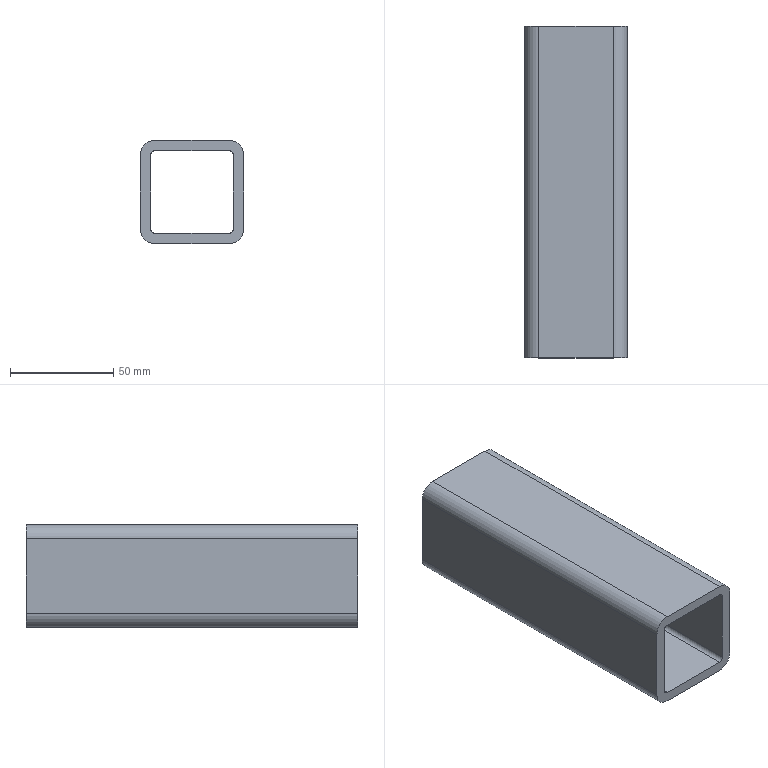Part | NX | 1 solid | 18 faces | box 50 x 161 x 50 mm | volume 138681 mm3 | plane 10 | cylinder 8 | commonest cylinder face diameters 4 x4 14 x4
STEP:
#1=CARTESIAN_POINT('',(305.,25.,393.));
#2=VERTEX_POINT('',#1);
#3=CARTESIAN_POINT('',(305.,186.,393.));
#4=VERTEX_POINT('',#3);
#5=CARTESIAN_POINT('',(305.,0.,393.));
#6=DIRECTION('',(0.,1.,0.));
#7=VECTOR('',#6,1000.);
#8=LINE('',#5,#7);
#9=EDGE_CURVE('',#2,#4,#8,.T.);
#10=ORIENTED_EDGE('',*,*,#9,.F.);
#11=CARTESIAN_POINT('',(305.,25.,357.));
#12=VERTEX_POINT('',#11);
#13=CARTESIAN_POINT('',(305.,25.,357.));
#14=DIRECTION('',(0.,0.,-1.));
#15=VECTOR('',#14,1000.);
#16=LINE('',#13,#15);
#17=EDGE_CURVE('',#2,#12,#16,.T.);
#18=ORIENTED_EDGE('',*,*,#17,.T.);
#19=CARTESIAN_POINT('',(305.,186.,357.));
#20=VERTEX_POINT('',#19);
#21=CARTESIAN_POINT('',(305.,0.,357.));
#22=DIRECTION('',(0.,1.,0.));
#23=VECTOR('',#22,1000.);
#24=LINE('',#21,#23);
#25=EDGE_CURVE('',#12,#20,#24,.T.);
#26=ORIENTED_EDGE('',*,*,#25,.T.);
#27=CARTESIAN_POINT('',(305.,186.,357.));
#28=DIRECTION('',(0.,0.,1.));
#29=VECTOR('',#28,1000.);
#30=LINE('',#27,#29);
#31=EDGE_CURVE('',#20,#4,#30,.T.);
#32=ORIENTED_EDGE('',*,*,#31,.T.);
#33=EDGE_LOOP('',(#10,#18,#26,#32));
#34=FACE_BOUND('',#33,.T.);
#35=CARTESIAN_POINT('',(305.,0.,357.));
#36=DIRECTION('',(1.,0.,0.));
#37=DIRECTION('',(0.,0.,-1.));
#38=AXIS2_PLACEMENT_3D('',#35,#36,#37);
#39=PLANE('',#38);
#40=ADVANCED_FACE('',(#34),#39,.T.);
#41=ORIENTED_EDGE('',*,*,#25,.F.);
#42=CARTESIAN_POINT('',(307.,25.,355.));
#43=VERTEX_POINT('',#42);
#44=CARTESIAN_POINT('',(307.,25.,357.));
#45=DIRECTION('',(0.,-1.,0.));
#46=DIRECTION('',(1.,0.,0.));
#47=AXIS2_PLACEMENT_3D('',#44,#45,#46);
#48=CIRCLE('',#47,2.);
#49=EDGE_CURVE('',#12,#43,#48,.T.);
#50=ORIENTED_EDGE('',*,*,#49,.T.);
#51=CARTESIAN_POINT('',(307.,186.,355.));
#52=VERTEX_POINT('',#51);
#53=CARTESIAN_POINT('',(307.,0.,355.));
#54=DIRECTION('',(0.,1.,0.));
#55=VECTOR('',#54,1000.);
#56=LINE('',#53,#55);
#57=EDGE_CURVE('',#43,#52,#56,.T.);
#58=ORIENTED_EDGE('',*,*,#57,.T.);
#59=CARTESIAN_POINT('',(307.,186.,357.));
#60=DIRECTION('',(0.,1.,0.));
#61=DIRECTION('',(-1.,0.,0.));
#62=AXIS2_PLACEMENT_3D('',#59,#60,#61);
#63=CIRCLE('',#62,2.);
#64=EDGE_CURVE('',#52,#20,#63,.T.);
#65=ORIENTED_EDGE('',*,*,#64,.T.);
#66=EDGE_LOOP('',(#41,#50,#58,#65));
#67=FACE_BOUND('',#66,.T.);
#68=CARTESIAN_POINT('',(307.,0.,357.));
#69=DIRECTION('',(0.,1.,0.));
#70=DIRECTION('',(0.,0.,1.));
#71=AXIS2_PLACEMENT_3D('',#68,#69,#70);
#72=CYLINDRICAL_SURFACE('',#71,2.);
#73=ADVANCED_FACE('',(#67),#72,.F.);
#74=ORIENTED_EDGE('',*,*,#57,.F.);
#75=CARTESIAN_POINT('',(343.,25.,355.));
#76=VERTEX_POINT('',#75);
#77=CARTESIAN_POINT('',(307.,25.,355.));
#78=DIRECTION('',(1.,0.,0.));
#79=VECTOR('',#78,1000.);
#80=LINE('',#77,#79);
#81=EDGE_CURVE('',#43,#76,#80,.T.);
#82=ORIENTED_EDGE('',*,*,#81,.T.);
#83=CARTESIAN_POINT('',(343.,186.,355.));
#84=VERTEX_POINT('',#83);
#85=CARTESIAN_POINT('',(343.,0.,355.));
#86=DIRECTION('',(0.,1.,0.));
#87=VECTOR('',#86,1000.);
#88=LINE('',#85,#87);
#89=EDGE_CURVE('',#76,#84,#88,.T.);
#90=ORIENTED_EDGE('',*,*,#89,.T.);
#91=CARTESIAN_POINT('',(307.,186.,355.));
#92=DIRECTION('',(-1.,0.,0.));
#93=VECTOR('',#92,1000.);
#94=LINE('',#91,#93);
#95=EDGE_CURVE('',#84,#52,#94,.T.);
#96=ORIENTED_EDGE('',*,*,#95,.T.);
#97=EDGE_LOOP('',(#74,#82,#90,#96));
#98=FACE_BOUND('',#97,.T.);
#99=CARTESIAN_POINT('',(307.,0.,355.));
#100=DIRECTION('',(0.,0.,1.));
#101=DIRECTION('',(0.,-1.,0.));
#102=AXIS2_PLACEMENT_3D('',#99,#100,#101);
#103=PLANE('',#102);
#104=ADVANCED_FACE('',(#98),#103,.T.);
#105=ORIENTED_EDGE('',*,*,#89,.F.);
#106=CARTESIAN_POINT('',(345.,25.,357.));
#107=VERTEX_POINT('',#106);
#108=CARTESIAN_POINT('',(343.,25.,357.));
#109=DIRECTION('',(0.,-1.,0.));
#110=DIRECTION('',(1.,0.,0.));
#111=AXIS2_PLACEMENT_3D('',#108,#109,#110);
#112=CIRCLE('',#111,2.);
#113=EDGE_CURVE('',#76,#107,#112,.T.);
#114=ORIENTED_EDGE('',*,*,#113,.T.);
#115=CARTESIAN_POINT('',(345.,186.,357.));
#116=VERTEX_POINT('',#115);
#117=CARTESIAN_POINT('',(345.,0.,357.));
#118=DIRECTION('',(0.,1.,0.));
#119=VECTOR('',#118,1000.);
#120=LINE('',#117,#119);
#121=EDGE_CURVE('',#107,#116,#120,.T.);
#122=ORIENTED_EDGE('',*,*,#121,.T.);
#123=CARTESIAN_POINT('',(343.,186.,357.));
#124=DIRECTION('',(0.,1.,0.));
#125=DIRECTION('',(-1.,0.,0.));
#126=AXIS2_PLACEMENT_3D('',#123,#124,#125);
#127=CIRCLE('',#126,2.);
#128=EDGE_CURVE('',#116,#84,#127,.T.);
#129=ORIENTED_EDGE('',*,*,#128,.T.);
#130=EDGE_LOOP('',(#105,#114,#122,#129));
#131=FACE_BOUND('',#130,.T.);
#132=CARTESIAN_POINT('',(343.,0.,357.));
#133=DIRECTION('',(0.,1.,0.));
#134=DIRECTION('',(0.,0.,1.));
#135=AXIS2_PLACEMENT_3D('',#132,#133,#134);
#136=CYLINDRICAL_SURFACE('',#135,2.);
#137=ADVANCED_FACE('',(#131),#136,.F.);
#138=ORIENTED_EDGE('',*,*,#121,.F.);
#139=CARTESIAN_POINT('',(345.,25.,393.));
#140=VERTEX_POINT('',#139);
#141=CARTESIAN_POINT('',(345.,25.,393.));
#142=DIRECTION('',(0.,0.,1.));
#143=VECTOR('',#142,1000.);
#144=LINE('',#141,#143);
#145=EDGE_CURVE('',#107,#140,#144,.T.);
#146=ORIENTED_EDGE('',*,*,#145,.T.);
#147=CARTESIAN_POINT('',(345.,186.,393.));
#148=VERTEX_POINT('',#147);
#149=CARTESIAN_POINT('',(345.,0.,393.));
#150=DIRECTION('',(0.,1.,0.));
#151=VECTOR('',#150,1000.);
#152=LINE('',#149,#151);
#153=EDGE_CURVE('',#140,#148,#152,.T.);
#154=ORIENTED_EDGE('',*,*,#153,.T.);
#155=CARTESIAN_POINT('',(345.,186.,393.));
#156=DIRECTION('',(0.,0.,-1.));
#157=VECTOR('',#156,1000.);
#158=LINE('',#155,#157);
#159=EDGE_CURVE('',#148,#116,#158,.T.);
#160=ORIENTED_EDGE('',*,*,#159,.T.);
#161=EDGE_LOOP('',(#138,#146,#154,#160));
#162=FACE_BOUND('',#161,.T.);
#163=CARTESIAN_POINT('',(345.,0.,393.));
#164=DIRECTION('',(-1.,0.,0.));
#165=DIRECTION('',(0.,0.,1.));
#166=AXIS2_PLACEMENT_3D('',#163,#164,#165);
#167=PLANE('',#166);
#168=ADVANCED_FACE('',(#162),#167,.T.);
#169=ORIENTED_EDGE('',*,*,#153,.F.);
#170=CARTESIAN_POINT('',(343.,25.,395.));
#171=VERTEX_POINT('',#170);
#172=CARTESIAN_POINT('',(343.,25.,393.));
#173=DIRECTION('',(0.,-1.,0.));
#174=DIRECTION('',(1.,0.,0.));
#175=AXIS2_PLACEMENT_3D('',#172,#173,#174);
#176=CIRCLE('',#175,2.);
#177=EDGE_CURVE('',#140,#171,#176,.T.);
#178=ORIENTED_EDGE('',*,*,#177,.T.);
#179=CARTESIAN_POINT('',(343.,186.,395.));
#180=VERTEX_POINT('',#179);
#181=CARTESIAN_POINT('',(343.,0.,395.));
#182=DIRECTION('',(0.,1.,0.));
#183=VECTOR('',#182,1000.);
#184=LINE('',#181,#183);
#185=EDGE_CURVE('',#171,#180,#184,.T.);
#186=ORIENTED_EDGE('',*,*,#185,.T.);
#187=CARTESIAN_POINT('',(343.,186.,393.));
#188=DIRECTION('',(0.,1.,0.));
#189=DIRECTION('',(-1.,0.,0.));
#190=AXIS2_PLACEMENT_3D('',#187,#188,#189);
#191=CIRCLE('',#190,2.);
#192=EDGE_CURVE('',#180,#148,#191,.T.);
#193=ORIENTED_EDGE('',*,*,#192,.T.);
#194=EDGE_LOOP('',(#169,#178,#186,#193));
#195=FACE_BOUND('',#194,.T.);
#196=CARTESIAN_POINT('',(343.,0.,393.));
#197=DIRECTION('',(0.,1.,0.));
#198=DIRECTION('',(0.,0.,1.));
#199=AXIS2_PLACEMENT_3D('',#196,#197,#198);
#200=CYLINDRICAL_SURFACE('',#199,2.);
#201=ADVANCED_FACE('',(#195),#200,.F.);
#202=ORIENTED_EDGE('',*,*,#185,.F.);
#203=CARTESIAN_POINT('',(307.,25.,395.));
#204=VERTEX_POINT('',#203);
#205=CARTESIAN_POINT('',(343.,25.,395.));
#206=DIRECTION('',(-1.,0.,0.));
#207=VECTOR('',#206,1000.);
#208=LINE('',#205,#207);
#209=EDGE_CURVE('',#171,#204,#208,.T.);
#210=ORIENTED_EDGE('',*,*,#209,.T.);
#211=CARTESIAN_POINT('',(307.,186.,395.));
#212=VERTEX_POINT('',#211);
#213=CARTESIAN_POINT('',(307.,0.,395.));
#214=DIRECTION('',(0.,1.,0.));
#215=VECTOR('',#214,1000.);
#216=LINE('',#213,#215);
#217=EDGE_CURVE('',#204,#212,#216,.T.);
#218=ORIENTED_EDGE('',*,*,#217,.T.);
#219=CARTESIAN_POINT('',(343.,186.,395.));
#220=DIRECTION('',(1.,0.,0.));
#221=VECTOR('',#220,1000.);
#222=LINE('',#219,#221);
#223=EDGE_CURVE('',#212,#180,#222,.T.);
#224=ORIENTED_EDGE('',*,*,#223,.T.);
#225=EDGE_LOOP('',(#202,#210,#218,#224));
#226=FACE_BOUND('',#225,.T.);
#227=CARTESIAN_POINT('',(343.,0.,395.));
#228=DIRECTION('',(0.,0.,-1.));
#229=DIRECTION('',(0.,1.,0.));
#230=AXIS2_PLACEMENT_3D('',#227,#228,#229);
#231=PLANE('',#230);
#232=ADVANCED_FACE('',(#226),#231,.T.);
#233=ORIENTED_EDGE('',*,*,#217,.F.);
#234=CARTESIAN_POINT('',(307.,25.,393.));
#235=DIRECTION('',(0.,-1.,0.));
#236=DIRECTION('',(1.,0.,0.));
#237=AXIS2_PLACEMENT_3D('',#234,#235,#236);
#238=CIRCLE('',#237,2.);
#239=EDGE_CURVE('',#204,#2,#238,.T.);
#240=ORIENTED_EDGE('',*,*,#239,.T.);
#241=ORIENTED_EDGE('',*,*,#9,.T.);
#242=CARTESIAN_POINT('',(307.,186.,393.));
#243=DIRECTION('',(0.,1.,0.));
#244=DIRECTION('',(-1.,0.,0.));
#245=AXIS2_PLACEMENT_3D('',#242,#243,#244);
#246=CIRCLE('',#245,2.);
#247=EDGE_CURVE('',#4,#212,#246,.T.);
#248=ORIENTED_EDGE('',*,*,#247,.T.);
#249=EDGE_LOOP('',(#233,#240,#241,#248));
#250=FACE_BOUND('',#249,.T.);
#251=CARTESIAN_POINT('',(307.,0.,393.));
#252=DIRECTION('',(0.,1.,0.));
#253=DIRECTION('',(0.,0.,1.));
#254=AXIS2_PLACEMENT_3D('',#251,#252,#253);
#255=CYLINDRICAL_SURFACE('',#254,2.);
#256=ADVANCED_FACE('',(#250),#255,.F.);
#257=CARTESIAN_POINT('',(350.,25.,393.));
#258=VERTEX_POINT('',#257);
#259=CARTESIAN_POINT('',(350.,186.,393.));
#260=VERTEX_POINT('',#259);
#261=CARTESIAN_POINT('',(350.,0.,393.));
#262=DIRECTION('',(0.,1.,0.));
#263=VECTOR('',#262,1000.);
#264=LINE('',#261,#263);
#265=EDGE_CURVE('',#258,#260,#264,.T.);
#266=ORIENTED_EDGE('',*,*,#265,.F.);
#267=CARTESIAN_POINT('',(350.,25.,357.));
#268=VERTEX_POINT('',#267);
#269=CARTESIAN_POINT('',(350.,25.,393.));
#270=DIRECTION('',(0.,0.,1.));
#271=VECTOR('',#270,1000.);
#272=LINE('',#269,#271);
#273=EDGE_CURVE('',#268,#258,#272,.T.);
#274=ORIENTED_EDGE('',*,*,#273,.F.);
#275=CARTESIAN_POINT('',(350.,186.,357.));
#276=VERTEX_POINT('',#275);
#277=CARTESIAN_POINT('',(350.,0.,357.));
#278=DIRECTION('',(0.,1.,0.));
#279=VECTOR('',#278,1000.);
#280=LINE('',#277,#279);
#281=EDGE_CURVE('',#268,#276,#280,.T.);
#282=ORIENTED_EDGE('',*,*,#281,.T.);
#283=CARTESIAN_POINT('',(350.,186.,393.));
#284=DIRECTION('',(0.,0.,-1.));
#285=VECTOR('',#284,1000.);
#286=LINE('',#283,#285);
#287=EDGE_CURVE('',#260,#276,#286,.T.);
#288=ORIENTED_EDGE('',*,*,#287,.F.);
#289=EDGE_LOOP('',(#266,#274,#282,#288));
#290=FACE_BOUND('',#289,.T.);
#291=CARTESIAN_POINT('',(350.,0.,393.));
#292=DIRECTION('',(-1.,0.,0.));
#293=DIRECTION('',(0.,0.,1.));
#294=AXIS2_PLACEMENT_3D('',#291,#292,#293);
#295=PLANE('',#294);
#296=ADVANCED_FACE('',(#290),#295,.F.);
#297=ORIENTED_EDGE('',*,*,#281,.F.);
#298=CARTESIAN_POINT('',(343.,25.,350.));
#299=VERTEX_POINT('',#298);
#300=CARTESIAN_POINT('',(343.,25.,357.));
#301=DIRECTION('',(0.,-1.,0.));
#302=DIRECTION('',(1.,0.,0.));
#303=AXIS2_PLACEMENT_3D('',#300,#301,#302);
#304=CIRCLE('',#303,7.);
#305=EDGE_CURVE('',#299,#268,#304,.T.);
#306=ORIENTED_EDGE('',*,*,#305,.F.);
#307=CARTESIAN_POINT('',(343.,186.,350.));
#308=VERTEX_POINT('',#307);
#309=CARTESIAN_POINT('',(343.,0.,350.));
#310=DIRECTION('',(0.,1.,0.));
#311=VECTOR('',#310,1000.);
#312=LINE('',#309,#311);
#313=EDGE_CURVE('',#299,#308,#312,.T.);
#314=ORIENTED_EDGE('',*,*,#313,.T.);
#315=CARTESIAN_POINT('',(343.,186.,357.));
#316=DIRECTION('',(0.,1.,0.));
#317=DIRECTION('',(-1.,0.,0.));
#318=AXIS2_PLACEMENT_3D('',#315,#316,#317);
#319=CIRCLE('',#318,7.);
#320=EDGE_CURVE('',#276,#308,#319,.T.);
#321=ORIENTED_EDGE('',*,*,#320,.F.);
#322=EDGE_LOOP('',(#297,#306,#314,#321));
#323=FACE_BOUND('',#322,.T.);
#324=CARTESIAN_POINT('',(343.,0.,357.));
#325=DIRECTION('',(0.,1.,0.));
#326=DIRECTION('',(0.,0.,1.));
#327=AXIS2_PLACEMENT_3D('',#324,#325,#326);
#328=CYLINDRICAL_SURFACE('',#327,7.);
#329=ADVANCED_FACE('',(#323),#328,.T.);
#330=ORIENTED_EDGE('',*,*,#313,.F.);
#331=CARTESIAN_POINT('',(307.,25.,350.));
#332=VERTEX_POINT('',#331);
#333=CARTESIAN_POINT('',(307.,25.,350.));
#334=DIRECTION('',(1.,0.,0.));
#335=VECTOR('',#334,1000.);
#336=LINE('',#333,#335);
#337=EDGE_CURVE('',#332,#299,#336,.T.);
#338=ORIENTED_EDGE('',*,*,#337,.F.);
#339=CARTESIAN_POINT('',(307.,186.,350.));
#340=VERTEX_POINT('',#339);
#341=CARTESIAN_POINT('',(307.,0.,350.));
#342=DIRECTION('',(0.,1.,0.));
#343=VECTOR('',#342,1000.);
#344=LINE('',#341,#343);
#345=EDGE_CURVE('',#332,#340,#344,.T.);
#346=ORIENTED_EDGE('',*,*,#345,.T.);
#347=CARTESIAN_POINT('',(307.,186.,350.));
#348=DIRECTION('',(-1.,0.,0.));
#349=VECTOR('',#348,1000.);
#350=LINE('',#347,#349);
#351=EDGE_CURVE('',#308,#340,#350,.T.);
#352=ORIENTED_EDGE('',*,*,#351,.F.);
#353=EDGE_LOOP('',(#330,#338,#346,#352));
#354=FACE_BOUND('',#353,.T.);
#355=CARTESIAN_POINT('',(307.,0.,350.));
#356=DIRECTION('',(0.,0.,1.));
#357=DIRECTION('',(0.,-1.,0.));
#358=AXIS2_PLACEMENT_3D('',#355,#356,#357);
#359=PLANE('',#358);
#360=ADVANCED_FACE('',(#354),#359,.F.);
#361=ORIENTED_EDGE('',*,*,#345,.F.);
#362=CARTESIAN_POINT('',(300.,25.,357.));
#363=VERTEX_POINT('',#362);
#364=CARTESIAN_POINT('',(307.,25.,357.));
#365=DIRECTION('',(0.,-1.,0.));
#366=DIRECTION('',(1.,0.,0.));
#367=AXIS2_PLACEMENT_3D('',#364,#365,#366);
#368=CIRCLE('',#367,7.);
#369=EDGE_CURVE('',#363,#332,#368,.T.);
#370=ORIENTED_EDGE('',*,*,#369,.F.);
#371=CARTESIAN_POINT('',(300.,186.,357.));
#372=VERTEX_POINT('',#371);
#373=CARTESIAN_POINT('',(300.,0.,357.));
#374=DIRECTION('',(0.,1.,0.));
#375=VECTOR('',#374,1000.);
#376=LINE('',#373,#375);
#377=EDGE_CURVE('',#363,#372,#376,.T.);
#378=ORIENTED_EDGE('',*,*,#377,.T.);
#379=CARTESIAN_POINT('',(307.,186.,357.));
#380=DIRECTION('',(0.,1.,0.));
#381=DIRECTION('',(-1.,0.,0.));
#382=AXIS2_PLACEMENT_3D('',#379,#380,#381);
#383=CIRCLE('',#382,7.);
#384=EDGE_CURVE('',#340,#372,#383,.T.);
#385=ORIENTED_EDGE('',*,*,#384,.F.);
#386=EDGE_LOOP('',(#361,#370,#378,#385));
#387=FACE_BOUND('',#386,.T.);
#388=CARTESIAN_POINT('',(307.,0.,357.));
#389=DIRECTION('',(0.,1.,0.));
#390=DIRECTION('',(0.,0.,1.));
#391=AXIS2_PLACEMENT_3D('',#388,#389,#390);
#392=CYLINDRICAL_SURFACE('',#391,7.);
#393=ADVANCED_FACE('',(#387),#392,.T.);
#394=ORIENTED_EDGE('',*,*,#377,.F.);
#395=CARTESIAN_POINT('',(300.,25.,393.));
#396=VERTEX_POINT('',#395);
#397=CARTESIAN_POINT('',(300.,25.,575.));
#398=DIRECTION('',(0.,0.,-1.));
#399=VECTOR('',#398,1000.);
#400=LINE('',#397,#399);
#401=EDGE_CURVE('',#396,#363,#400,.T.);
#402=ORIENTED_EDGE('',*,*,#401,.F.);
#403=CARTESIAN_POINT('',(300.,186.,393.));
#404=VERTEX_POINT('',#403);
#405=CARTESIAN_POINT('',(300.,0.,393.));
#406=DIRECTION('',(0.,1.,0.));
#407=VECTOR('',#406,1000.);
#408=LINE('',#405,#407);
#409=EDGE_CURVE('',#396,#404,#408,.T.);
#410=ORIENTED_EDGE('',*,*,#409,.T.);
#411=CARTESIAN_POINT('',(300.,186.,357.));
#412=DIRECTION('',(0.,0.,1.));
#413=VECTOR('',#412,1000.);
#414=LINE('',#411,#413);
#415=EDGE_CURVE('',#372,#404,#414,.T.);
#416=ORIENTED_EDGE('',*,*,#415,.F.);
#417=EDGE_LOOP('',(#394,#402,#410,#416));
#418=FACE_BOUND('',#417,.T.);
#419=CARTESIAN_POINT('',(300.,0.,357.));
#420=DIRECTION('',(1.,0.,0.));
#421=DIRECTION('',(0.,0.,-1.));
#422=AXIS2_PLACEMENT_3D('',#419,#420,#421);
#423=PLANE('',#422);
#424=ADVANCED_FACE('',(#418),#423,.F.);
#425=ORIENTED_EDGE('',*,*,#409,.F.);
#426=CARTESIAN_POINT('',(307.,25.,400.));
#427=VERTEX_POINT('',#426);
#428=CARTESIAN_POINT('',(307.,25.,393.));
#429=DIRECTION('',(0.,-1.,0.));
#430=DIRECTION('',(1.,0.,0.));
#431=AXIS2_PLACEMENT_3D('',#428,#429,#430);
#432=CIRCLE('',#431,7.);
#433=EDGE_CURVE('',#427,#396,#432,.T.);
#434=ORIENTED_EDGE('',*,*,#433,.F.);
#435=CARTESIAN_POINT('',(307.,186.,400.));
#436=VERTEX_POINT('',#435);
#437=CARTESIAN_POINT('',(307.,0.,400.));
#438=DIRECTION('',(0.,1.,0.));
#439=VECTOR('',#438,1000.);
#440=LINE('',#437,#439);
#441=EDGE_CURVE('',#427,#436,#440,.T.);
#442=ORIENTED_EDGE('',*,*,#441,.T.);
#443=CARTESIAN_POINT('',(307.,186.,393.));
#444=DIRECTION('',(0.,1.,0.));
#445=DIRECTION('',(-1.,0.,0.));
#446=AXIS2_PLACEMENT_3D('',#443,#444,#445);
#447=CIRCLE('',#446,7.);
#448=EDGE_CURVE('',#404,#436,#447,.T.);
#449=ORIENTED_EDGE('',*,*,#448,.F.);
#450=EDGE_LOOP('',(#425,#434,#442,#449));
#451=FACE_BOUND('',#450,.T.);
#452=CARTESIAN_POINT('',(307.,0.,393.));
#453=DIRECTION('',(0.,1.,0.));
#454=DIRECTION('',(0.,0.,1.));
#455=AXIS2_PLACEMENT_3D('',#452,#453,#454);
#456=CYLINDRICAL_SURFACE('',#455,7.);
#457=ADVANCED_FACE('',(#451),#456,.T.);
#458=ORIENTED_EDGE('',*,*,#441,.F.);
#459=CARTESIAN_POINT('',(343.,25.,400.));
#460=VERTEX_POINT('',#459);
#461=CARTESIAN_POINT('',(343.,25.,400.));
#462=DIRECTION('',(-1.,0.,0.));
#463=VECTOR('',#462,1000.);
#464=LINE('',#461,#463);
#465=EDGE_CURVE('',#460,#427,#464,.T.);
#466=ORIENTED_EDGE('',*,*,#465,.F.);
#467=CARTESIAN_POINT('',(343.,186.,400.));
#468=VERTEX_POINT('',#467);
#469=CARTESIAN_POINT('',(343.,0.,400.));
#470=DIRECTION('',(0.,1.,0.));
#471=VECTOR('',#470,1000.);
#472=LINE('',#469,#471);
#473=EDGE_CURVE('',#460,#468,#472,.T.);
#474=ORIENTED_EDGE('',*,*,#473,.T.);
#475=CARTESIAN_POINT('',(343.,186.,400.));
#476=DIRECTION('',(1.,0.,0.));
#477=VECTOR('',#476,1000.);
#478=LINE('',#475,#477);
#479=EDGE_CURVE('',#436,#468,#478,.T.);
#480=ORIENTED_EDGE('',*,*,#479,.F.);
#481=EDGE_LOOP('',(#458,#466,#474,#480));
#482=FACE_BOUND('',#481,.T.);
#483=CARTESIAN_POINT('',(343.,0.,400.));
#484=DIRECTION('',(0.,0.,-1.));
#485=DIRECTION('',(0.,1.,0.));
#486=AXIS2_PLACEMENT_3D('',#483,#484,#485);
#487=PLANE('',#486);
#488=ADVANCED_FACE('',(#482),#487,.F.);
#489=ORIENTED_EDGE('',*,*,#473,.F.);
#490=CARTESIAN_POINT('',(343.,25.,393.));
#491=DIRECTION('',(0.,-1.,0.));
#492=DIRECTION('',(1.,0.,0.));
#493=AXIS2_PLACEMENT_3D('',#490,#491,#492);
#494=CIRCLE('',#493,7.);
#495=EDGE_CURVE('',#258,#460,#494,.T.);
#496=ORIENTED_EDGE('',*,*,#495,.F.);
#497=ORIENTED_EDGE('',*,*,#265,.T.);
#498=CARTESIAN_POINT('',(343.,186.,393.));
#499=DIRECTION('',(0.,1.,0.));
#500=DIRECTION('',(-1.,0.,0.));
#501=AXIS2_PLACEMENT_3D('',#498,#499,#500);
#502=CIRCLE('',#501,7.);
#503=EDGE_CURVE('',#468,#260,#502,.T.);
#504=ORIENTED_EDGE('',*,*,#503,.F.);
#505=EDGE_LOOP('',(#489,#496,#497,#504));
#506=FACE_BOUND('',#505,.T.);
#507=CARTESIAN_POINT('',(343.,0.,393.));
#508=DIRECTION('',(0.,1.,0.));
#509=DIRECTION('',(0.,0.,1.));
#510=AXIS2_PLACEMENT_3D('',#507,#508,#509);
#511=CYLINDRICAL_SURFACE('',#510,7.);
#512=ADVANCED_FACE('',(#506),#511,.T.);
#513=ORIENTED_EDGE('',*,*,#31,.F.);
#514=ORIENTED_EDGE('',*,*,#64,.F.);
#515=ORIENTED_EDGE('',*,*,#95,.F.);
#516=ORIENTED_EDGE('',*,*,#128,.F.);
#517=ORIENTED_EDGE('',*,*,#159,.F.);
#518=ORIENTED_EDGE('',*,*,#192,.F.);
#519=ORIENTED_EDGE('',*,*,#223,.F.);
#520=ORIENTED_EDGE('',*,*,#247,.F.);
#521=EDGE_LOOP('',(#513,#514,#515,#516,#517,#518,#519,#520));
#522=FACE_BOUND('',#521,.T.);
#523=ORIENTED_EDGE('',*,*,#503,.T.);
#524=ORIENTED_EDGE('',*,*,#287,.T.);
#525=ORIENTED_EDGE('',*,*,#320,.T.);
#526=ORIENTED_EDGE('',*,*,#351,.T.);
#527=ORIENTED_EDGE('',*,*,#384,.T.);
#528=ORIENTED_EDGE('',*,*,#415,.T.);
#529=ORIENTED_EDGE('',*,*,#448,.T.);
#530=ORIENTED_EDGE('',*,*,#479,.T.);
#531=EDGE_LOOP('',(#523,#524,#525,#526,#527,#528,#529,#530));
#532=FACE_BOUND('',#531,.T.);
#533=CARTESIAN_POINT('',(975.,186.,0.));
#534=DIRECTION('',(0.,1.,0.));
#535=DIRECTION('',(-1.,0.,0.));
#536=AXIS2_PLACEMENT_3D('',#533,#534,#535);
#537=PLANE('',#536);
#538=ADVANCED_FACE('',(#522,#532),#537,.T.);
#539=ORIENTED_EDGE('',*,*,#209,.F.);
#540=ORIENTED_EDGE('',*,*,#177,.F.);
#541=ORIENTED_EDGE('',*,*,#145,.F.);
#542=ORIENTED_EDGE('',*,*,#113,.F.);
#543=ORIENTED_EDGE('',*,*,#81,.F.);
#544=ORIENTED_EDGE('',*,*,#49,.F.);
#545=ORIENTED_EDGE('',*,*,#17,.F.);
#546=ORIENTED_EDGE('',*,*,#239,.F.);
#547=EDGE_LOOP('',(#539,#540,#541,#542,#543,#544,#545,#546));
#548=FACE_BOUND('',#547,.T.);
#549=ORIENTED_EDGE('',*,*,#495,.T.);
#550=ORIENTED_EDGE('',*,*,#465,.T.);
#551=ORIENTED_EDGE('',*,*,#433,.T.);
#552=ORIENTED_EDGE('',*,*,#401,.T.);
#553=ORIENTED_EDGE('',*,*,#369,.T.);
#554=ORIENTED_EDGE('',*,*,#337,.T.);
#555=ORIENTED_EDGE('',*,*,#305,.T.);
#556=ORIENTED_EDGE('',*,*,#273,.T.);
#557=EDGE_LOOP('',(#549,#550,#551,#552,#553,#554,#555,#556));
#558=FACE_BOUND('',#557,.T.);
#559=CARTESIAN_POINT('',(343.,25.,575.));
#560=DIRECTION('',(0.,-1.,0.));
#561=DIRECTION('',(1.,0.,0.));
#562=AXIS2_PLACEMENT_3D('',#559,#560,#561);
#563=PLANE('',#562);
#564=ADVANCED_FACE('',(#548,#558),#563,.T.);
#565=CLOSED_SHELL('',(#40,#73,#104,#137,#168,#201,#232,#256,#296,#329,#360,#393,#424,#457,#488,#512,#538,#564));
#566=MANIFOLD_SOLID_BREP('',#565);
#567=(LENGTH_UNIT()NAMED_UNIT(*)SI_UNIT(.MILLI.,.METRE.));
#568=UNCERTAINTY_MEASURE_WITH_UNIT(LENGTH_MEASURE(0.00001),#567,'','');
#569=(NAMED_UNIT(*)PLANE_ANGLE_UNIT()SI_UNIT($,.RADIAN.));
#570=(NAMED_UNIT(*)SI_UNIT($,.STERADIAN.)SOLID_ANGLE_UNIT());
#571=(GEOMETRIC_REPRESENTATION_CONTEXT(3)GLOBAL_UNCERTAINTY_ASSIGNED_CONTEXT((#568))GLOBAL_UNIT_ASSIGNED_CONTEXT((#567,#569,#570))REPRESENTATION_CONTEXT('',''));
#572=ADVANCED_BREP_SHAPE_REPRESENTATION('',(#566),#571);